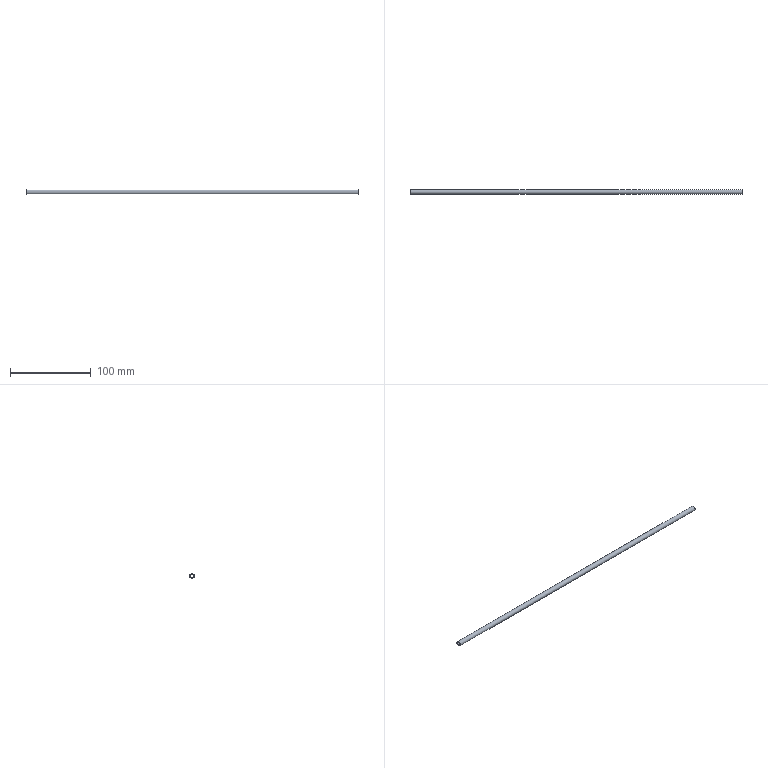Part | NX | features solid 2 | 1 solid | 4 faces | box 410 x 6 x 6 mm | volume 6440 mm3 | cylinder 2 | plane 2 | commonest cylinder face diameters 4 x1 6 x1
STEP:
#1=CARTESIAN_POINT('',(520.,-54.,347.));
#2=VERTEX_POINT('',#1);
#3=CARTESIAN_POINT('',(520.,-52.,347.));
#4=DIRECTION('',(-1.,0.,0.));
#5=DIRECTION('',(0.,-1.,0.));
#6=AXIS2_PLACEMENT_3D('',#3,#4,#5);
#7=CIRCLE('',#6,2.);
#8=EDGE_CURVE('',#2,#2,#7,.T.);
#9=ORIENTED_EDGE('',*,*,#8,.F.);
#10=EDGE_LOOP('',(#9));
#11=FACE_BOUND('',#10,.T.);
#12=CARTESIAN_POINT('',(110.,-54.,347.));
#13=VERTEX_POINT('',#12);
#14=CARTESIAN_POINT('',(110.,-52.,347.));
#15=DIRECTION('',(-1.,0.,0.));
#16=DIRECTION('',(0.,-1.,0.));
#17=AXIS2_PLACEMENT_3D('',#14,#15,#16);
#18=CIRCLE('',#17,2.);
#19=EDGE_CURVE('',#13,#13,#18,.T.);
#20=ORIENTED_EDGE('',*,*,#19,.T.);
#21=EDGE_LOOP('',(#20));
#22=FACE_BOUND('',#21,.T.);
#23=CARTESIAN_POINT('',(241.176,-52.,347.));
#24=DIRECTION('',(1.,0.,0.));
#25=DIRECTION('',(0.,1.,0.));
#26=AXIS2_PLACEMENT_3D('',#23,#24,#25);
#27=CYLINDRICAL_SURFACE('',#26,2.);
#28=ADVANCED_FACE('',(#11,#22),#27,.F.);
#29=CARTESIAN_POINT('',(520.,-55.,347.));
#30=VERTEX_POINT('',#29);
#31=CARTESIAN_POINT('',(520.,-52.,347.));
#32=DIRECTION('',(-1.,0.,0.));
#33=DIRECTION('',(0.,-1.,0.));
#34=AXIS2_PLACEMENT_3D('',#31,#32,#33);
#35=CIRCLE('',#34,3.);
#36=EDGE_CURVE('',#30,#30,#35,.T.);
#37=ORIENTED_EDGE('',*,*,#36,.T.);
#38=EDGE_LOOP('',(#37));
#39=FACE_BOUND('',#38,.T.);
#40=CARTESIAN_POINT('',(110.,-55.,347.));
#41=VERTEX_POINT('',#40);
#42=CARTESIAN_POINT('',(110.,-52.,347.));
#43=DIRECTION('',(-1.,0.,0.));
#44=DIRECTION('',(0.,-1.,0.));
#45=AXIS2_PLACEMENT_3D('',#42,#43,#44);
#46=CIRCLE('',#45,3.);
#47=EDGE_CURVE('',#41,#41,#46,.T.);
#48=ORIENTED_EDGE('',*,*,#47,.F.);
#49=EDGE_LOOP('',(#48));
#50=FACE_BOUND('',#49,.T.);
#51=CARTESIAN_POINT('',(241.176,-52.,347.));
#52=DIRECTION('',(1.,0.,0.));
#53=DIRECTION('',(0.,1.,0.));
#54=AXIS2_PLACEMENT_3D('',#51,#52,#53);
#55=CYLINDRICAL_SURFACE('',#54,3.);
#56=ADVANCED_FACE('',(#39,#50),#55,.T.);
#57=ORIENTED_EDGE('',*,*,#8,.T.);
#58=EDGE_LOOP('',(#57));
#59=FACE_BOUND('',#58,.T.);
#60=ORIENTED_EDGE('',*,*,#36,.F.);
#61=EDGE_LOOP('',(#60));
#62=FACE_BOUND('',#61,.T.);
#63=CARTESIAN_POINT('',(520.,-52.,347.));
#64=DIRECTION('',(-1.,0.,0.));
#65=DIRECTION('',(0.,-1.,0.));
#66=AXIS2_PLACEMENT_3D('',#63,#64,#65);
#67=PLANE('',#66);
#68=ADVANCED_FACE('',(#59,#62),#67,.F.);
#69=ORIENTED_EDGE('',*,*,#19,.F.);
#70=EDGE_LOOP('',(#69));
#71=FACE_BOUND('',#70,.T.);
#72=ORIENTED_EDGE('',*,*,#47,.T.);
#73=EDGE_LOOP('',(#72));
#74=FACE_BOUND('',#73,.T.);
#75=CARTESIAN_POINT('',(110.,35.,347.));
#76=DIRECTION('',(-1.,0.,0.));
#77=DIRECTION('',(0.,-1.,0.));
#78=AXIS2_PLACEMENT_3D('',#75,#76,#77);
#79=PLANE('',#78);
#80=ADVANCED_FACE('',(#71,#74),#79,.T.);
#81=CLOSED_SHELL('',(#28,#56,#68,#80));
#82=MANIFOLD_SOLID_BREP('',#81);
#83=(LENGTH_UNIT()NAMED_UNIT(*)SI_UNIT(.MILLI.,.METRE.));
#84=UNCERTAINTY_MEASURE_WITH_UNIT(LENGTH_MEASURE(0.00001),#83,'','');
#85=(NAMED_UNIT(*)PLANE_ANGLE_UNIT()SI_UNIT($,.RADIAN.));
#86=(NAMED_UNIT(*)SI_UNIT($,.STERADIAN.)SOLID_ANGLE_UNIT());
#87=(GEOMETRIC_REPRESENTATION_CONTEXT(3)GLOBAL_UNCERTAINTY_ASSIGNED_CONTEXT((#84))GLOBAL_UNIT_ASSIGNED_CONTEXT((#83,#85,#86))REPRESENTATION_CONTEXT('',''));
#88=ADVANCED_BREP_SHAPE_REPRESENTATION('',(#82),#87);